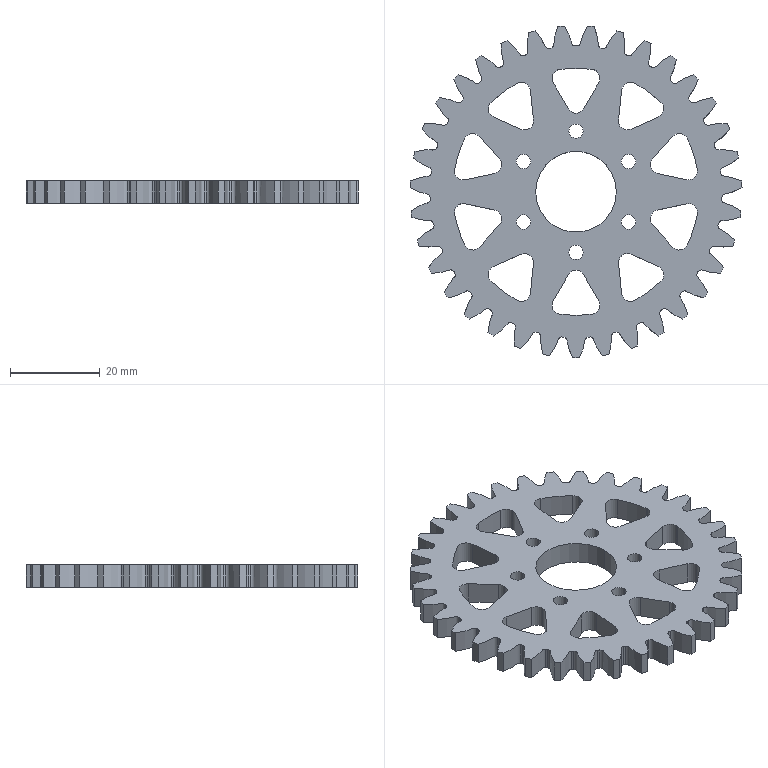Part | SolidWorks | features ICE 3, CirPattern 1, Extrusion 1, RefAxis 1 | 1 solid | 226 faces | box 73.978 x 73.911 x 5 mm | volume 13896 mm3 | cylinder 134 | spline 70 | plane 22 | commonest cylinder face diameters 4 x40 65 x35 74 x35 3.2 x12 55 x10 18 x2